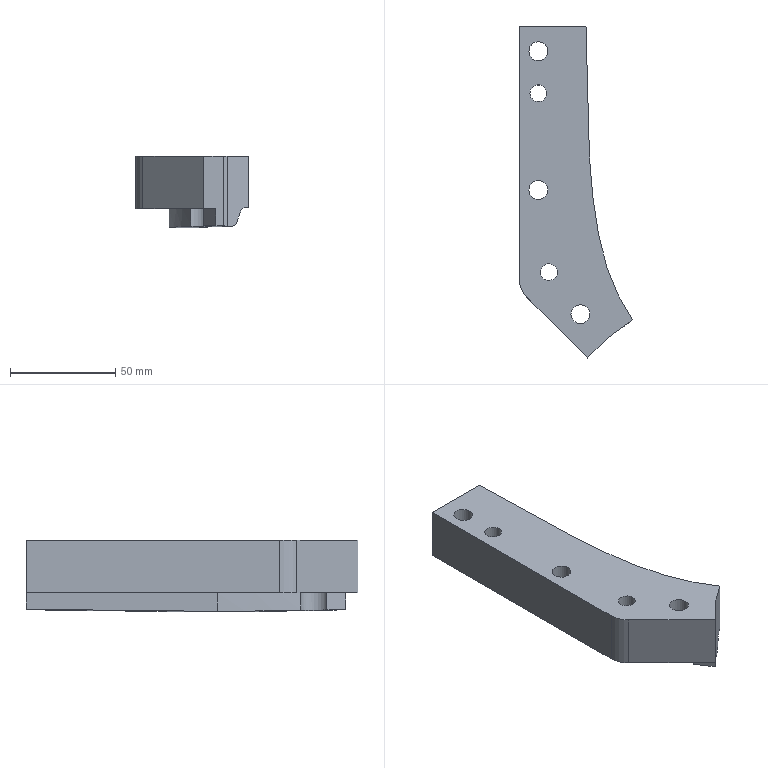Part | STEP file | 812_id1590_x_t | 1 solid | 44 faces | box 53.803 x 157.778 x 34.221 mm | volume 136586 mm3 | spline 19 | plane 13 | cylinder 12 | commonest cylinder face diameters 9 x3 14 x3 8 x2 10 x2 24 x1 30 x1